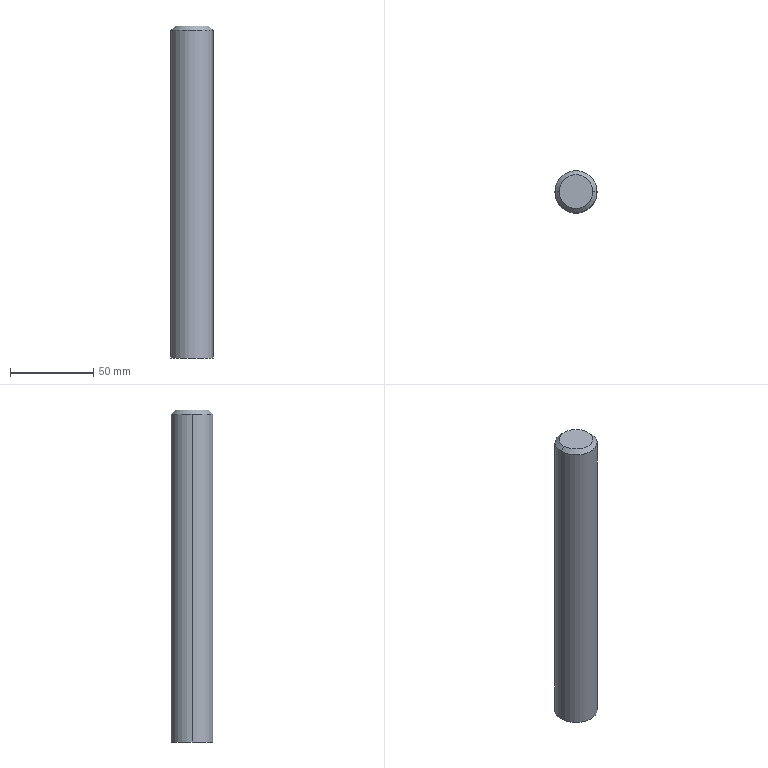Part | SolidWorks | features Chamfer 1, Extrusion 1, Scale 1 | 1 solid | 6 faces | box 25.4 x 25.4 x 200 mm | volume 101101 mm3 | cone 2 | cylinder 2 | plane 2 | commonest cylinder face diameters 25.4 x2
STEP:
#1=CARTESIAN_POINT('',(10.16,0.,0.));
#2=VERTEX_POINT('',#1);
#3=CARTESIAN_POINT('',(-10.16,0.,0.));
#4=VERTEX_POINT('',#3);
#5=CARTESIAN_POINT('',(0.,0.,0.));
#6=DIRECTION('',(0.,0.,1.));
#7=DIRECTION('',(1.,0.,0.));
#8=AXIS2_PLACEMENT_3D('',#5,#6,#7);
#9=CIRCLE('',#8,10.16);
#10=EDGE_CURVE('',#2,#4,#9,.T.);
#11=ORIENTED_EDGE('',*,*,#10,.F.);
#12=CARTESIAN_POINT('',(12.7,0.,-2.54));
#13=VERTEX_POINT('',#12);
#14=CARTESIAN_POINT('',(10.16,0.,0.));
#15=DIRECTION('',(0.7071,0.,-0.7071));
#16=VECTOR('',#15,1000.);
#17=LINE('',#14,#16);
#18=EDGE_CURVE('',#2,#13,#17,.T.);
#19=ORIENTED_EDGE('',*,*,#18,.T.);
#20=CARTESIAN_POINT('',(-12.7,0.,-2.54));
#21=VERTEX_POINT('',#20);
#22=CARTESIAN_POINT('',(0.,0.,-2.54));
#23=DIRECTION('',(0.,0.,-1.));
#24=DIRECTION('',(1.,0.,0.));
#25=AXIS2_PLACEMENT_3D('',#22,#23,#24);
#26=CIRCLE('',#25,12.7);
#27=EDGE_CURVE('',#21,#13,#26,.T.);
#28=ORIENTED_EDGE('',*,*,#27,.F.);
#29=CARTESIAN_POINT('',(-10.16,0.,0.));
#30=DIRECTION('',(-0.7071,0.,-0.7071));
#31=VECTOR('',#30,1000.);
#32=LINE('',#29,#31);
#33=EDGE_CURVE('',#4,#21,#32,.T.);
#34=ORIENTED_EDGE('',*,*,#33,.F.);
#35=EDGE_LOOP('',(#11,#19,#28,#34));
#36=FACE_OUTER_BOUND('',#35,.T.);
#37=CARTESIAN_POINT('',(0.,0.,0.));
#38=DIRECTION('',(0.,0.,-1.));
#39=DIRECTION('',(-1.,0.,0.));
#40=AXIS2_PLACEMENT_3D('',#37,#38,#39);
#41=CONICAL_SURFACE('',#40,10.16,0.7854);
#42=ADVANCED_FACE('',(#36),#41,.T.);
#43=CARTESIAN_POINT('',(12.7,0.,-200.));
#44=VERTEX_POINT('',#43);
#45=CARTESIAN_POINT('',(-12.7,0.,-200.));
#46=VERTEX_POINT('',#45);
#47=CARTESIAN_POINT('',(0.,0.,-200.));
#48=DIRECTION('',(0.,0.,1.));
#49=DIRECTION('',(1.,0.,0.));
#50=AXIS2_PLACEMENT_3D('',#47,#48,#49);
#51=CIRCLE('',#50,12.7);
#52=EDGE_CURVE('',#44,#46,#51,.T.);
#53=ORIENTED_EDGE('',*,*,#52,.T.);
#54=CARTESIAN_POINT('',(-12.7,0.,-200.));
#55=DIRECTION('',(0.,0.,1.));
#56=VECTOR('',#55,1000.);
#57=LINE('',#54,#56);
#58=EDGE_CURVE('',#46,#21,#57,.T.);
#59=ORIENTED_EDGE('',*,*,#58,.T.);
#60=ORIENTED_EDGE('',*,*,#27,.T.);
#61=CARTESIAN_POINT('',(12.7,0.,-200.));
#62=DIRECTION('',(0.,0.,1.));
#63=VECTOR('',#62,1000.);
#64=LINE('',#61,#63);
#65=EDGE_CURVE('',#44,#13,#64,.T.);
#66=ORIENTED_EDGE('',*,*,#65,.F.);
#67=EDGE_LOOP('',(#53,#59,#60,#66));
#68=FACE_OUTER_BOUND('',#67,.T.);
#69=CARTESIAN_POINT('',(0.,0.,-200.));
#70=DIRECTION('',(0.,0.,1.));
#71=DIRECTION('',(1.,0.,0.));
#72=AXIS2_PLACEMENT_3D('',#69,#70,#71);
#73=CYLINDRICAL_SURFACE('',#72,12.7);
#74=ADVANCED_FACE('',(#68),#73,.T.);
#75=ORIENTED_EDGE('',*,*,#58,.F.);
#76=CARTESIAN_POINT('',(0.,0.,-200.));
#77=DIRECTION('',(0.,0.,1.));
#78=DIRECTION('',(1.,0.,0.));
#79=AXIS2_PLACEMENT_3D('',#76,#77,#78);
#80=CIRCLE('',#79,12.7);
#81=EDGE_CURVE('',#46,#44,#80,.T.);
#82=ORIENTED_EDGE('',*,*,#81,.T.);
#83=ORIENTED_EDGE('',*,*,#65,.T.);
#84=CARTESIAN_POINT('',(0.,0.,-2.54));
#85=DIRECTION('',(0.,0.,-1.));
#86=DIRECTION('',(1.,0.,0.));
#87=AXIS2_PLACEMENT_3D('',#84,#85,#86);
#88=CIRCLE('',#87,12.7);
#89=EDGE_CURVE('',#13,#21,#88,.T.);
#90=ORIENTED_EDGE('',*,*,#89,.T.);
#91=EDGE_LOOP('',(#75,#82,#83,#90));
#92=FACE_OUTER_BOUND('',#91,.T.);
#93=CARTESIAN_POINT('',(0.,0.,-200.));
#94=DIRECTION('',(0.,0.,1.));
#95=DIRECTION('',(1.,0.,0.));
#96=AXIS2_PLACEMENT_3D('',#93,#94,#95);
#97=CYLINDRICAL_SURFACE('',#96,12.7);
#98=ADVANCED_FACE('',(#92),#97,.T.);
#99=ORIENTED_EDGE('',*,*,#52,.F.);
#100=ORIENTED_EDGE('',*,*,#81,.F.);
#101=EDGE_LOOP('',(#99,#100));
#102=FACE_OUTER_BOUND('',#101,.T.);
#103=CARTESIAN_POINT('',(0.,0.,-200.));
#104=DIRECTION('',(0.,0.,1.));
#105=DIRECTION('',(1.,0.,0.));
#106=AXIS2_PLACEMENT_3D('',#103,#104,#105);
#107=PLANE('',#106);
#108=ADVANCED_FACE('',(#102),#107,.F.);
#109=CARTESIAN_POINT('',(0.,0.,0.));
#110=DIRECTION('',(0.,0.,1.));
#111=DIRECTION('',(1.,0.,0.));
#112=AXIS2_PLACEMENT_3D('',#109,#110,#111);
#113=CIRCLE('',#112,10.16);
#114=EDGE_CURVE('',#4,#2,#113,.T.);
#115=ORIENTED_EDGE('',*,*,#114,.T.);
#116=ORIENTED_EDGE('',*,*,#10,.T.);
#117=EDGE_LOOP('',(#115,#116));
#118=FACE_OUTER_BOUND('',#117,.T.);
#119=CARTESIAN_POINT('',(0.,0.,0.));
#120=DIRECTION('',(0.,0.,1.));
#121=DIRECTION('',(1.,0.,0.));
#122=AXIS2_PLACEMENT_3D('',#119,#120,#121);
#123=PLANE('',#122);
#124=ADVANCED_FACE('',(#118),#123,.T.);
#125=ORIENTED_EDGE('',*,*,#18,.F.);
#126=ORIENTED_EDGE('',*,*,#114,.F.);
#127=ORIENTED_EDGE('',*,*,#33,.T.);
#128=ORIENTED_EDGE('',*,*,#89,.F.);
#129=EDGE_LOOP('',(#125,#126,#127,#128));
#130=FACE_OUTER_BOUND('',#129,.T.);
#131=CARTESIAN_POINT('',(0.,0.,0.));
#132=DIRECTION('',(0.,0.,-1.));
#133=DIRECTION('',(-1.,0.,0.));
#134=AXIS2_PLACEMENT_3D('',#131,#132,#133);
#135=CONICAL_SURFACE('',#134,10.16,0.7854);
#136=ADVANCED_FACE('',(#130),#135,.T.);
#137=CLOSED_SHELL('',(#42,#74,#98,#108,#124,#136));
#138=MANIFOLD_SOLID_BREP('',#137);
#139=CARTESIAN_POINT('',(0.,0.,0.));
#140=DIRECTION('',(0.,0.,1.));
#141=DIRECTION('',(1.,0.,0.));
#142=AXIS2_PLACEMENT_3D('',#139,#140,#141);
#143=(LENGTH_UNIT()NAMED_UNIT(*)SI_UNIT(.MILLI.,.METRE.));
#144=UNCERTAINTY_MEASURE_WITH_UNIT(LENGTH_MEASURE(0.00001),#143,'','');
#145=(NAMED_UNIT(*)PLANE_ANGLE_UNIT()SI_UNIT($,.RADIAN.));
#146=(NAMED_UNIT(*)SI_UNIT($,.STERADIAN.)SOLID_ANGLE_UNIT());
#147=(GEOMETRIC_REPRESENTATION_CONTEXT(3)GLOBAL_UNCERTAINTY_ASSIGNED_CONTEXT((#144))GLOBAL_UNIT_ASSIGNED_CONTEXT((#143,#145,#146))REPRESENTATION_CONTEXT('',''));
#148=ADVANCED_BREP_SHAPE_REPRESENTATION('',(#138,#142),#147);